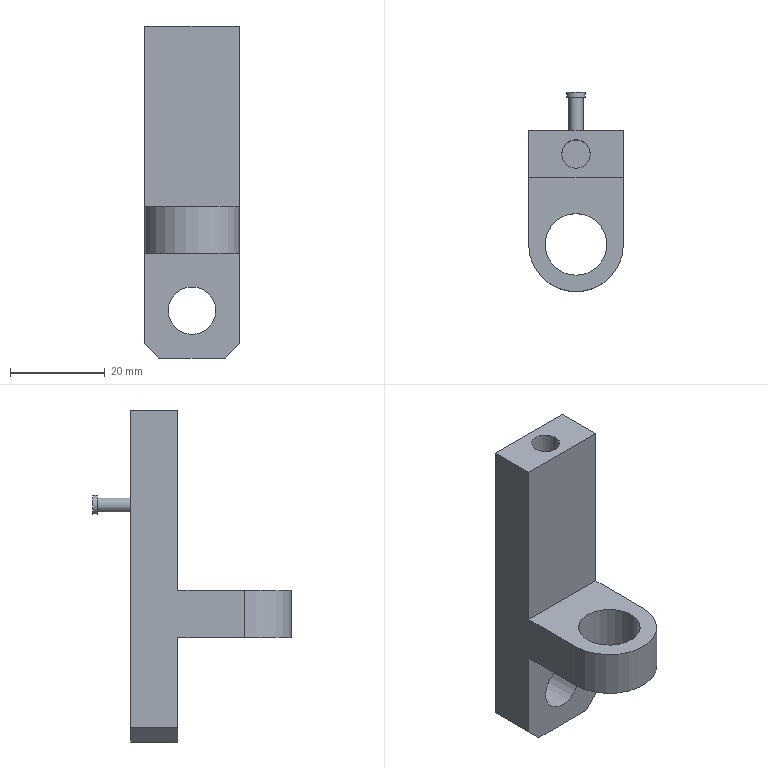Part | NX | features DATUM_CSYS 5, EXTRUDE 4, SKETCH 4, HOLE PACKAGE 1, SIMPLE HOLE 1 | 1 solid | 20 faces | box 20 x 42 x 70 mm | volume 14816 mm3 | plane 14 | cylinder 6 | commonest cylinder face diameters 3 x1 4 x1 6 x1 10 x1 13 x1 20 x1
STEP:
#1=CARTESIAN_POINT('',(5.,-5.,-60.));
#2=VERTEX_POINT('',#1);
#3=CARTESIAN_POINT('',(0.,-5.,-60.));
#4=DIRECTION('',(0.,-1.,0.));
#5=DIRECTION('',(1.,0.,0.));
#6=AXIS2_PLACEMENT_3D('',#3,#4,#5);
#7=CIRCLE('',#6,5.);
#8=EDGE_CURVE('',#2,#2,#7,.T.);
#9=ORIENTED_EDGE('',*,*,#8,.F.);
#10=EDGE_LOOP('',(#9));
#11=FACE_BOUND('',#10,.T.);
#12=CARTESIAN_POINT('',(10.,-5.,-67.));
#13=VERTEX_POINT('',#12);
#14=CARTESIAN_POINT('',(10.,-5.,-48.));
#15=VERTEX_POINT('',#14);
#16=CARTESIAN_POINT('',(10.,-5.,-67.));
#17=DIRECTION('',(0.,0.,1.));
#18=VECTOR('',#17,1000.);
#19=LINE('',#16,#18);
#20=EDGE_CURVE('',#13,#15,#19,.T.);
#21=ORIENTED_EDGE('',*,*,#20,.T.);
#22=CARTESIAN_POINT('',(-10.,-5.,-48.));
#23=VERTEX_POINT('',#22);
#24=CARTESIAN_POINT('',(10.,-5.,-48.));
#25=DIRECTION('',(-1.,0.,0.));
#26=VECTOR('',#25,1000.);
#27=LINE('',#24,#26);
#28=EDGE_CURVE('',#15,#23,#27,.T.);
#29=ORIENTED_EDGE('',*,*,#28,.T.);
#30=CARTESIAN_POINT('',(-10.,-5.,-67.));
#31=VERTEX_POINT('',#30);
#32=CARTESIAN_POINT('',(-10.,-5.,0.));
#33=DIRECTION('',(0.,0.,-1.));
#34=VECTOR('',#33,1000.);
#35=LINE('',#32,#34);
#36=EDGE_CURVE('',#23,#31,#35,.T.);
#37=ORIENTED_EDGE('',*,*,#36,.T.);
#38=CARTESIAN_POINT('',(-7.,-5.,-70.));
#39=VERTEX_POINT('',#38);
#40=CARTESIAN_POINT('',(-10.,-5.,-67.));
#41=DIRECTION('',(0.7071,0.,-0.7071));
#42=VECTOR('',#41,1000.);
#43=LINE('',#40,#42);
#44=EDGE_CURVE('',#31,#39,#43,.T.);
#45=ORIENTED_EDGE('',*,*,#44,.T.);
#46=CARTESIAN_POINT('',(7.,-5.,-70.));
#47=VERTEX_POINT('',#46);
#48=CARTESIAN_POINT('',(-7.,-5.,-70.));
#49=DIRECTION('',(1.,0.,0.));
#50=VECTOR('',#49,1000.);
#51=LINE('',#48,#50);
#52=EDGE_CURVE('',#39,#47,#51,.T.);
#53=ORIENTED_EDGE('',*,*,#52,.T.);
#54=CARTESIAN_POINT('',(7.,-5.,-70.));
#55=DIRECTION('',(0.7071,0.,0.7071));
#56=VECTOR('',#55,1000.);
#57=LINE('',#54,#56);
#58=EDGE_CURVE('',#47,#13,#57,.T.);
#59=ORIENTED_EDGE('',*,*,#58,.T.);
#60=EDGE_LOOP('',(#21,#29,#37,#45,#53,#59));
#61=FACE_BOUND('',#60,.T.);
#62=CARTESIAN_POINT('',(0.,-5.,-60.));
#63=DIRECTION('',(0.,-1.,0.));
#64=DIRECTION('',(0.,0.,-1.));
#65=AXIS2_PLACEMENT_3D('',#62,#63,#64);
#66=PLANE('',#65);
#67=ADVANCED_FACE('',(#11,#61),#66,.T.);
#68=CARTESIAN_POINT('',(-10.,5.,0.));
#69=VERTEX_POINT('',#68);
#70=CARTESIAN_POINT('',(-10.,5.,-67.));
#71=VERTEX_POINT('',#70);
#72=CARTESIAN_POINT('',(-10.,5.,0.));
#73=DIRECTION('',(0.,0.,-1.));
#74=VECTOR('',#73,1000.);
#75=LINE('',#72,#74);
#76=EDGE_CURVE('',#69,#71,#75,.T.);
#77=ORIENTED_EDGE('',*,*,#76,.T.);
#78=CARTESIAN_POINT('',(-10.,-5.,-67.));
#79=DIRECTION('',(0.,1.,0.));
#80=VECTOR('',#79,1000.);
#81=LINE('',#78,#80);
#82=EDGE_CURVE('',#31,#71,#81,.T.);
#83=ORIENTED_EDGE('',*,*,#82,.F.);
#84=ORIENTED_EDGE('',*,*,#36,.F.);
#85=CARTESIAN_POINT('',(-10.,-19.,-48.));
#86=VERTEX_POINT('',#85);
#87=CARTESIAN_POINT('',(-10.,-5.,-48.));
#88=DIRECTION('',(0.,-1.,0.));
#89=VECTOR('',#88,1000.);
#90=LINE('',#87,#89);
#91=EDGE_CURVE('',#23,#86,#90,.T.);
#92=ORIENTED_EDGE('',*,*,#91,.T.);
#93=CARTESIAN_POINT('',(-10.,-19.,-38.));
#94=VERTEX_POINT('',#93);
#95=CARTESIAN_POINT('',(-10.,-19.,-48.));
#96=DIRECTION('',(0.,0.,1.));
#97=VECTOR('',#96,1000.);
#98=LINE('',#95,#97);
#99=EDGE_CURVE('',#86,#94,#98,.T.);
#100=ORIENTED_EDGE('',*,*,#99,.T.);
#101=CARTESIAN_POINT('',(-10.,-5.,-38.));
#102=VERTEX_POINT('',#101);
#103=CARTESIAN_POINT('',(-10.,-5.,-38.));
#104=DIRECTION('',(0.,-1.,0.));
#105=VECTOR('',#104,1000.);
#106=LINE('',#103,#105);
#107=EDGE_CURVE('',#102,#94,#106,.T.);
#108=ORIENTED_EDGE('',*,*,#107,.F.);
#109=CARTESIAN_POINT('',(-10.,-5.,0.));
#110=VERTEX_POINT('',#109);
#111=CARTESIAN_POINT('',(-10.,-5.,0.));
#112=DIRECTION('',(0.,0.,-1.));
#113=VECTOR('',#112,1000.);
#114=LINE('',#111,#113);
#115=EDGE_CURVE('',#110,#102,#114,.T.);
#116=ORIENTED_EDGE('',*,*,#115,.F.);
#117=CARTESIAN_POINT('',(-10.,-5.,0.));
#118=DIRECTION('',(0.,1.,0.));
#119=VECTOR('',#118,1000.);
#120=LINE('',#117,#119);
#121=EDGE_CURVE('',#110,#69,#120,.T.);
#122=ORIENTED_EDGE('',*,*,#121,.T.);
#123=EDGE_LOOP('',(#77,#83,#84,#92,#100,#108,#116,#122));
#124=FACE_BOUND('',#123,.T.);
#125=CARTESIAN_POINT('',(-10.,-5.,0.));
#126=DIRECTION('',(1.,0.,0.));
#127=DIRECTION('',(0.,0.,-1.));
#128=AXIS2_PLACEMENT_3D('',#125,#126,#127);
#129=PLANE('',#128);
#130=ADVANCED_FACE('',(#124),#129,.F.);
#131=CARTESIAN_POINT('',(-7.,5.,-70.));
#132=VERTEX_POINT('',#131);
#133=CARTESIAN_POINT('',(-10.,5.,-67.));
#134=DIRECTION('',(0.7071,0.,-0.7071));
#135=VECTOR('',#134,1000.);
#136=LINE('',#133,#135);
#137=EDGE_CURVE('',#71,#132,#136,.T.);
#138=ORIENTED_EDGE('',*,*,#137,.T.);
#139=CARTESIAN_POINT('',(-7.,-5.,-70.));
#140=DIRECTION('',(0.,1.,0.));
#141=VECTOR('',#140,1000.);
#142=LINE('',#139,#141);
#143=EDGE_CURVE('',#39,#132,#142,.T.);
#144=ORIENTED_EDGE('',*,*,#143,.F.);
#145=ORIENTED_EDGE('',*,*,#44,.F.);
#146=ORIENTED_EDGE('',*,*,#82,.T.);
#147=EDGE_LOOP('',(#138,#144,#145,#146));
#148=FACE_BOUND('',#147,.T.);
#149=CARTESIAN_POINT('',(-10.,-5.,-67.));
#150=DIRECTION('',(0.7071,0.,0.7071));
#151=DIRECTION('',(0.7071,0.,-0.7071));
#152=AXIS2_PLACEMENT_3D('',#149,#150,#151);
#153=PLANE('',#152);
#154=ADVANCED_FACE('',(#148),#153,.F.);
#155=CARTESIAN_POINT('',(7.,5.,-70.));
#156=VERTEX_POINT('',#155);
#157=CARTESIAN_POINT('',(-7.,5.,-70.));
#158=DIRECTION('',(1.,0.,0.));
#159=VECTOR('',#158,1000.);
#160=LINE('',#157,#159);
#161=EDGE_CURVE('',#132,#156,#160,.T.);
#162=ORIENTED_EDGE('',*,*,#161,.T.);
#163=CARTESIAN_POINT('',(7.,-5.,-70.));
#164=DIRECTION('',(0.,1.,0.));
#165=VECTOR('',#164,1000.);
#166=LINE('',#163,#165);
#167=EDGE_CURVE('',#47,#156,#166,.T.);
#168=ORIENTED_EDGE('',*,*,#167,.F.);
#169=ORIENTED_EDGE('',*,*,#52,.F.);
#170=ORIENTED_EDGE('',*,*,#143,.T.);
#171=EDGE_LOOP('',(#162,#168,#169,#170));
#172=FACE_BOUND('',#171,.T.);
#173=CARTESIAN_POINT('',(-7.,-5.,-70.));
#174=DIRECTION('',(0.,0.,1.));
#175=DIRECTION('',(1.,0.,0.));
#176=AXIS2_PLACEMENT_3D('',#173,#174,#175);
#177=PLANE('',#176);
#178=ADVANCED_FACE('',(#172),#177,.F.);
#179=CARTESIAN_POINT('',(10.,5.,-67.));
#180=VERTEX_POINT('',#179);
#181=CARTESIAN_POINT('',(7.,5.,-70.));
#182=DIRECTION('',(0.7071,0.,0.7071));
#183=VECTOR('',#182,1000.);
#184=LINE('',#181,#183);
#185=EDGE_CURVE('',#156,#180,#184,.T.);
#186=ORIENTED_EDGE('',*,*,#185,.T.);
#187=CARTESIAN_POINT('',(10.,-5.,-67.));
#188=DIRECTION('',(0.,1.,0.));
#189=VECTOR('',#188,1000.);
#190=LINE('',#187,#189);
#191=EDGE_CURVE('',#13,#180,#190,.T.);
#192=ORIENTED_EDGE('',*,*,#191,.F.);
#193=ORIENTED_EDGE('',*,*,#58,.F.);
#194=ORIENTED_EDGE('',*,*,#167,.T.);
#195=EDGE_LOOP('',(#186,#192,#193,#194));
#196=FACE_BOUND('',#195,.T.);
#197=CARTESIAN_POINT('',(7.,-5.,-70.));
#198=DIRECTION('',(-0.7071,0.,0.7071));
#199=DIRECTION('',(0.7071,0.,0.7071));
#200=AXIS2_PLACEMENT_3D('',#197,#198,#199);
#201=PLANE('',#200);
#202=ADVANCED_FACE('',(#196),#201,.F.);
#203=CARTESIAN_POINT('',(10.,5.,0.));
#204=VERTEX_POINT('',#203);
#205=CARTESIAN_POINT('',(10.,5.,-67.));
#206=DIRECTION('',(0.,0.,1.));
#207=VECTOR('',#206,1000.);
#208=LINE('',#205,#207);
#209=EDGE_CURVE('',#180,#204,#208,.T.);
#210=ORIENTED_EDGE('',*,*,#209,.T.);
#211=CARTESIAN_POINT('',(10.,-5.,0.));
#212=VERTEX_POINT('',#211);
#213=CARTESIAN_POINT('',(10.,-5.,0.));
#214=DIRECTION('',(0.,1.,0.));
#215=VECTOR('',#214,1000.);
#216=LINE('',#213,#215);
#217=EDGE_CURVE('',#212,#204,#216,.T.);
#218=ORIENTED_EDGE('',*,*,#217,.F.);
#219=CARTESIAN_POINT('',(10.,-5.,-38.));
#220=VERTEX_POINT('',#219);
#221=CARTESIAN_POINT('',(10.,-5.,-67.));
#222=DIRECTION('',(0.,0.,1.));
#223=VECTOR('',#222,1000.);
#224=LINE('',#221,#223);
#225=EDGE_CURVE('',#220,#212,#224,.T.);
#226=ORIENTED_EDGE('',*,*,#225,.F.);
#227=CARTESIAN_POINT('',(10.,-19.,-38.));
#228=VERTEX_POINT('',#227);
#229=CARTESIAN_POINT('',(10.,-19.,-38.));
#230=DIRECTION('',(0.,1.,0.));
#231=VECTOR('',#230,1000.);
#232=LINE('',#229,#231);
#233=EDGE_CURVE('',#228,#220,#232,.T.);
#234=ORIENTED_EDGE('',*,*,#233,.F.);
#235=CARTESIAN_POINT('',(10.,-19.,-48.));
#236=VERTEX_POINT('',#235);
#237=CARTESIAN_POINT('',(10.,-19.,-48.));
#238=DIRECTION('',(0.,0.,1.));
#239=VECTOR('',#238,1000.);
#240=LINE('',#237,#239);
#241=EDGE_CURVE('',#236,#228,#240,.T.);
#242=ORIENTED_EDGE('',*,*,#241,.F.);
#243=CARTESIAN_POINT('',(10.,-19.,-48.));
#244=DIRECTION('',(0.,1.,0.));
#245=VECTOR('',#244,1000.);
#246=LINE('',#243,#245);
#247=EDGE_CURVE('',#236,#15,#246,.T.);
#248=ORIENTED_EDGE('',*,*,#247,.T.);
#249=ORIENTED_EDGE('',*,*,#20,.F.);
#250=ORIENTED_EDGE('',*,*,#191,.T.);
#251=EDGE_LOOP('',(#210,#218,#226,#234,#242,#248,#249,#250));
#252=FACE_BOUND('',#251,.T.);
#253=CARTESIAN_POINT('',(10.,-5.,-67.));
#254=DIRECTION('',(-1.,0.,0.));
#255=DIRECTION('',(0.,0.,1.));
#256=AXIS2_PLACEMENT_3D('',#253,#254,#255);
#257=PLANE('',#256);
#258=ADVANCED_FACE('',(#252),#257,.F.);
#259=CARTESIAN_POINT('',(-3.,0.,0.));
#260=VERTEX_POINT('',#259);
#261=CARTESIAN_POINT('',(0.,0.,0.));
#262=DIRECTION('',(0.,0.,-1.));
#263=DIRECTION('',(-1.,0.,0.));
#264=AXIS2_PLACEMENT_3D('',#261,#262,#263);
#265=CIRCLE('',#264,3.);
#266=EDGE_CURVE('',#260,#260,#265,.T.);
#267=ORIENTED_EDGE('',*,*,#266,.T.);
#268=EDGE_LOOP('',(#267));
#269=FACE_BOUND('',#268,.T.);
#270=CARTESIAN_POINT('',(10.,5.,0.));
#271=DIRECTION('',(-1.,0.,0.));
#272=VECTOR('',#271,1000.);
#273=LINE('',#270,#272);
#274=EDGE_CURVE('',#204,#69,#273,.T.);
#275=ORIENTED_EDGE('',*,*,#274,.T.);
#276=ORIENTED_EDGE('',*,*,#121,.F.);
#277=CARTESIAN_POINT('',(10.,-5.,0.));
#278=DIRECTION('',(-1.,0.,0.));
#279=VECTOR('',#278,1000.);
#280=LINE('',#277,#279);
#281=EDGE_CURVE('',#212,#110,#280,.T.);
#282=ORIENTED_EDGE('',*,*,#281,.F.);
#283=ORIENTED_EDGE('',*,*,#217,.T.);
#284=EDGE_LOOP('',(#275,#276,#282,#283));
#285=FACE_BOUND('',#284,.T.);
#286=CARTESIAN_POINT('',(10.,-5.,0.));
#287=DIRECTION('',(0.,0.,-1.));
#288=DIRECTION('',(-1.,0.,0.));
#289=AXIS2_PLACEMENT_3D('',#286,#287,#288);
#290=PLANE('',#289);
#291=ADVANCED_FACE('',(#269,#285),#290,.F.);
#292=ORIENTED_EDGE('',*,*,#8,.T.);
#293=EDGE_LOOP('',(#292));
#294=FACE_BOUND('',#293,.T.);
#295=CARTESIAN_POINT('',(5.,5.,-60.));
#296=VERTEX_POINT('',#295);
#297=CARTESIAN_POINT('',(0.,5.,-60.));
#298=DIRECTION('',(0.,-1.,0.));
#299=DIRECTION('',(1.,0.,0.));
#300=AXIS2_PLACEMENT_3D('',#297,#298,#299);
#301=CIRCLE('',#300,5.);
#302=EDGE_CURVE('',#296,#296,#301,.T.);
#303=ORIENTED_EDGE('',*,*,#302,.F.);
#304=EDGE_LOOP('',(#303));
#305=FACE_BOUND('',#304,.T.);
#306=CARTESIAN_POINT('',(0.,-5.,-60.));
#307=DIRECTION('',(0.,1.,0.));
#308=DIRECTION('',(0.,0.,1.));
#309=AXIS2_PLACEMENT_3D('',#306,#307,#308);
#310=CYLINDRICAL_SURFACE('',#309,5.);
#311=ADVANCED_FACE('',(#294,#305),#310,.F.);
#312=CARTESIAN_POINT('',(10.,-5.,-38.));
#313=DIRECTION('',(-1.,0.,0.));
#314=VECTOR('',#313,1000.);
#315=LINE('',#312,#314);
#316=EDGE_CURVE('',#220,#102,#315,.T.);
#317=ORIENTED_EDGE('',*,*,#316,.F.);
#318=ORIENTED_EDGE('',*,*,#225,.T.);
#319=ORIENTED_EDGE('',*,*,#281,.T.);
#320=ORIENTED_EDGE('',*,*,#115,.T.);
#321=EDGE_LOOP('',(#317,#318,#319,#320));
#322=FACE_BOUND('',#321,.T.);
#323=CARTESIAN_POINT('',(0.,-5.,-60.));
#324=DIRECTION('',(0.,-1.,0.));
#325=DIRECTION('',(0.,0.,-1.));
#326=AXIS2_PLACEMENT_3D('',#323,#324,#325);
#327=PLANE('',#326);
#328=ADVANCED_FACE('',(#322),#327,.T.);
#329=CARTESIAN_POINT('',(1.5,5.,-20.));
#330=VERTEX_POINT('',#329);
#331=CARTESIAN_POINT('',(0.,5.,-20.));
#332=DIRECTION('',(0.,-1.,0.));
#333=DIRECTION('',(1.,0.,0.));
#334=AXIS2_PLACEMENT_3D('',#331,#332,#333);
#335=CIRCLE('',#334,1.5);
#336=EDGE_CURVE('',#330,#330,#335,.T.);
#337=ORIENTED_EDGE('',*,*,#336,.T.);
#338=EDGE_LOOP('',(#337));
#339=FACE_BOUND('',#338,.T.);
#340=ORIENTED_EDGE('',*,*,#76,.F.);
#341=ORIENTED_EDGE('',*,*,#274,.F.);
#342=ORIENTED_EDGE('',*,*,#209,.F.);
#343=ORIENTED_EDGE('',*,*,#185,.F.);
#344=ORIENTED_EDGE('',*,*,#161,.F.);
#345=ORIENTED_EDGE('',*,*,#137,.F.);
#346=EDGE_LOOP('',(#340,#341,#342,#343,#344,#345));
#347=FACE_BOUND('',#346,.T.);
#348=ORIENTED_EDGE('',*,*,#302,.T.);
#349=EDGE_LOOP('',(#348));
#350=FACE_BOUND('',#349,.T.);
#351=CARTESIAN_POINT('',(0.,5.,-60.));
#352=DIRECTION('',(0.,-1.,0.));
#353=DIRECTION('',(0.,0.,-1.));
#354=AXIS2_PLACEMENT_3D('',#351,#352,#353);
#355=PLANE('',#354);
#356=ADVANCED_FACE('',(#339,#347,#350),#355,.F.);
#357=CARTESIAN_POINT('',(1.5,12.,-20.));
#358=VERTEX_POINT('',#357);
#359=CARTESIAN_POINT('',(0.,12.,-20.));
#360=DIRECTION('',(0.,-1.,0.));
#361=DIRECTION('',(1.,0.,0.));
#362=AXIS2_PLACEMENT_3D('',#359,#360,#361);
#363=CIRCLE('',#362,1.5);
#364=EDGE_CURVE('',#358,#358,#363,.T.);
#365=ORIENTED_EDGE('',*,*,#364,.T.);
#366=EDGE_LOOP('',(#365));
#367=FACE_BOUND('',#366,.T.);
#368=ORIENTED_EDGE('',*,*,#336,.F.);
#369=EDGE_LOOP('',(#368));
#370=FACE_BOUND('',#369,.T.);
#371=CARTESIAN_POINT('',(0.,12.,-20.));
#372=DIRECTION('',(0.,-1.,0.));
#373=DIRECTION('',(0.,0.,-1.));
#374=AXIS2_PLACEMENT_3D('',#371,#372,#373);
#375=CYLINDRICAL_SURFACE('',#374,1.5);
#376=ADVANCED_FACE('',(#367,#370),#375,.T.);
#377=CARTESIAN_POINT('',(-2.,13.,-20.));
#378=VERTEX_POINT('',#377);
#379=CARTESIAN_POINT('',(0.,13.,-20.));
#380=DIRECTION('',(0.,-1.,0.));
#381=DIRECTION('',(-1.,0.,0.));
#382=AXIS2_PLACEMENT_3D('',#379,#380,#381);
#383=CIRCLE('',#382,2.);
#384=EDGE_CURVE('',#378,#378,#383,.T.);
#385=ORIENTED_EDGE('',*,*,#384,.T.);
#386=EDGE_LOOP('',(#385));
#387=FACE_BOUND('',#386,.T.);
#388=CARTESIAN_POINT('',(-2.,12.,-20.));
#389=VERTEX_POINT('',#388);
#390=CARTESIAN_POINT('',(0.,12.,-20.));
#391=DIRECTION('',(0.,-1.,0.));
#392=DIRECTION('',(-1.,0.,0.));
#393=AXIS2_PLACEMENT_3D('',#390,#391,#392);
#394=CIRCLE('',#393,2.);
#395=EDGE_CURVE('',#389,#389,#394,.T.);
#396=ORIENTED_EDGE('',*,*,#395,.F.);
#397=EDGE_LOOP('',(#396));
#398=FACE_BOUND('',#397,.T.);
#399=CARTESIAN_POINT('',(0.,13.,-20.));
#400=DIRECTION('',(0.,-1.,0.));
#401=DIRECTION('',(0.,0.,-1.));
#402=AXIS2_PLACEMENT_3D('',#399,#400,#401);
#403=CYLINDRICAL_SURFACE('',#402,2.);
#404=ADVANCED_FACE('',(#387,#398),#403,.T.);
#405=ORIENTED_EDGE('',*,*,#384,.F.);
#406=EDGE_LOOP('',(#405));
#407=FACE_BOUND('',#406,.T.);
#408=CARTESIAN_POINT('',(0.,13.,-20.));
#409=DIRECTION('',(0.,-1.,0.));
#410=DIRECTION('',(0.,0.,-1.));
#411=AXIS2_PLACEMENT_3D('',#408,#409,#410);
#412=PLANE('',#411);
#413=ADVANCED_FACE('',(#407),#412,.F.);
#414=ORIENTED_EDGE('',*,*,#364,.F.);
#415=EDGE_LOOP('',(#414));
#416=FACE_BOUND('',#415,.T.);
#417=ORIENTED_EDGE('',*,*,#395,.T.);
#418=EDGE_LOOP('',(#417));
#419=FACE_BOUND('',#418,.T.);
#420=CARTESIAN_POINT('',(0.,12.,-20.));
#421=DIRECTION('',(0.,-1.,0.));
#422=DIRECTION('',(0.,0.,-1.));
#423=AXIS2_PLACEMENT_3D('',#420,#421,#422);
#424=PLANE('',#423);
#425=ADVANCED_FACE('',(#416,#419),#424,.T.);
#426=CARTESIAN_POINT('',(-3.,0.,-50.));
#427=VERTEX_POINT('',#426);
#428=CARTESIAN_POINT('',(0.,0.,-50.));
#429=DIRECTION('',(0.,0.,-1.));
#430=DIRECTION('',(-1.,0.,0.));
#431=AXIS2_PLACEMENT_3D('',#428,#429,#430);
#432=CIRCLE('',#431,3.);
#433=EDGE_CURVE('',#427,#427,#432,.F.);
#434=ORIENTED_EDGE('',*,*,#433,.T.);
#435=EDGE_LOOP('',(#434));
#436=FACE_BOUND('',#435,.T.);
#437=CARTESIAN_POINT('',(0.,0.,-50.));
#438=DIRECTION('',(0.,0.,-1.));
#439=DIRECTION('',(-1.,0.,0.));
#440=AXIS2_PLACEMENT_3D('',#437,#438,#439);
#441=PLANE('',#440);
#442=ADVANCED_FACE('',(#436),#441,.F.);
#443=ORIENTED_EDGE('',*,*,#433,.F.);
#444=EDGE_LOOP('',(#443));
#445=FACE_BOUND('',#444,.T.);
#446=ORIENTED_EDGE('',*,*,#266,.F.);
#447=EDGE_LOOP('',(#446));
#448=FACE_BOUND('',#447,.T.);
#449=CARTESIAN_POINT('',(0.,0.,0.));
#450=DIRECTION('',(0.,0.,-1.));
#451=DIRECTION('',(-1.,0.,0.));
#452=AXIS2_PLACEMENT_3D('',#449,#450,#451);
#453=CYLINDRICAL_SURFACE('',#452,3.);
#454=ADVANCED_FACE('',(#445,#448),#453,.F.);
#455=CARTESIAN_POINT('',(0.,-19.,-38.));
#456=DIRECTION('',(0.,0.,1.));
#457=DIRECTION('',(0.,-1.,0.));
#458=AXIS2_PLACEMENT_3D('',#455,#456,#457);
#459=CIRCLE('',#458,10.);
#460=EDGE_CURVE('',#94,#228,#459,.T.);
#461=ORIENTED_EDGE('',*,*,#460,.F.);
#462=ORIENTED_EDGE('',*,*,#99,.F.);
#463=CARTESIAN_POINT('',(0.,-19.,-48.));
#464=DIRECTION('',(0.,0.,1.));
#465=DIRECTION('',(0.,-1.,0.));
#466=AXIS2_PLACEMENT_3D('',#463,#464,#465);
#467=CIRCLE('',#466,10.);
#468=EDGE_CURVE('',#86,#236,#467,.T.);
#469=ORIENTED_EDGE('',*,*,#468,.T.);
#470=ORIENTED_EDGE('',*,*,#241,.T.);
#471=EDGE_LOOP('',(#461,#462,#469,#470));
#472=FACE_BOUND('',#471,.T.);
#473=CARTESIAN_POINT('',(0.,-19.,-48.));
#474=DIRECTION('',(0.,0.,1.));
#475=DIRECTION('',(1.,0.,0.));
#476=AXIS2_PLACEMENT_3D('',#473,#474,#475);
#477=CYLINDRICAL_SURFACE('',#476,10.);
#478=ADVANCED_FACE('',(#472),#477,.T.);
#479=CARTESIAN_POINT('',(0.,-12.5,-48.));
#480=VERTEX_POINT('',#479);
#481=CARTESIAN_POINT('',(0.,-19.,-48.));
#482=DIRECTION('',(0.,0.,-1.));
#483=DIRECTION('',(0.,1.,0.));
#484=AXIS2_PLACEMENT_3D('',#481,#482,#483);
#485=CIRCLE('',#484,6.5);
#486=EDGE_CURVE('',#480,#480,#485,.T.);
#487=ORIENTED_EDGE('',*,*,#486,.T.);
#488=EDGE_LOOP('',(#487));
#489=FACE_BOUND('',#488,.T.);
#490=CARTESIAN_POINT('',(0.,-12.5,-38.));
#491=VERTEX_POINT('',#490);
#492=CARTESIAN_POINT('',(0.,-19.,-38.));
#493=DIRECTION('',(0.,0.,-1.));
#494=DIRECTION('',(0.,1.,0.));
#495=AXIS2_PLACEMENT_3D('',#492,#493,#494);
#496=CIRCLE('',#495,6.5);
#497=EDGE_CURVE('',#491,#491,#496,.T.);
#498=ORIENTED_EDGE('',*,*,#497,.F.);
#499=EDGE_LOOP('',(#498));
#500=FACE_BOUND('',#499,.T.);
#501=CARTESIAN_POINT('',(0.,-19.,-48.));
#502=DIRECTION('',(0.,0.,1.));
#503=DIRECTION('',(1.,0.,0.));
#504=AXIS2_PLACEMENT_3D('',#501,#502,#503);
#505=CYLINDRICAL_SURFACE('',#504,6.5);
#506=ADVANCED_FACE('',(#489,#500),#505,.F.);
#507=ORIENTED_EDGE('',*,*,#91,.F.);
#508=ORIENTED_EDGE('',*,*,#28,.F.);
#509=ORIENTED_EDGE('',*,*,#247,.F.);
#510=ORIENTED_EDGE('',*,*,#468,.F.);
#511=EDGE_LOOP('',(#507,#508,#509,#510));
#512=FACE_BOUND('',#511,.T.);
#513=ORIENTED_EDGE('',*,*,#486,.F.);
#514=EDGE_LOOP('',(#513));
#515=FACE_BOUND('',#514,.T.);
#516=CARTESIAN_POINT('',(0.,-19.,-48.));
#517=DIRECTION('',(0.,0.,1.));
#518=DIRECTION('',(1.,0.,0.));
#519=AXIS2_PLACEMENT_3D('',#516,#517,#518);
#520=PLANE('',#519);
#521=ADVANCED_FACE('',(#512,#515),#520,.F.);
#522=ORIENTED_EDGE('',*,*,#107,.T.);
#523=ORIENTED_EDGE('',*,*,#460,.T.);
#524=ORIENTED_EDGE('',*,*,#233,.T.);
#525=ORIENTED_EDGE('',*,*,#316,.T.);
#526=EDGE_LOOP('',(#522,#523,#524,#525));
#527=FACE_BOUND('',#526,.T.);
#528=ORIENTED_EDGE('',*,*,#497,.T.);
#529=EDGE_LOOP('',(#528));
#530=FACE_BOUND('',#529,.T.);
#531=CARTESIAN_POINT('',(0.,-19.,-38.));
#532=DIRECTION('',(0.,0.,1.));
#533=DIRECTION('',(1.,0.,0.));
#534=AXIS2_PLACEMENT_3D('',#531,#532,#533);
#535=PLANE('',#534);
#536=ADVANCED_FACE('',(#527,#530),#535,.T.);
#537=CLOSED_SHELL('',(#67,#130,#154,#178,#202,#258,#291,#311,#328,#356,#376,#404,#413,#425,#442,#454,#478,#506,#521,#536));
#538=MANIFOLD_SOLID_BREP('',#537);
#539=(LENGTH_UNIT()NAMED_UNIT(*)SI_UNIT(.MILLI.,.METRE.));
#540=UNCERTAINTY_MEASURE_WITH_UNIT(LENGTH_MEASURE(0.00001),#539,'','');
#541=(NAMED_UNIT(*)PLANE_ANGLE_UNIT()SI_UNIT($,.RADIAN.));
#542=(NAMED_UNIT(*)SI_UNIT($,.STERADIAN.)SOLID_ANGLE_UNIT());
#543=(GEOMETRIC_REPRESENTATION_CONTEXT(3)GLOBAL_UNCERTAINTY_ASSIGNED_CONTEXT((#540))GLOBAL_UNIT_ASSIGNED_CONTEXT((#539,#541,#542))REPRESENTATION_CONTEXT('',''));
#544=ADVANCED_BREP_SHAPE_REPRESENTATION('',(#538),#543);